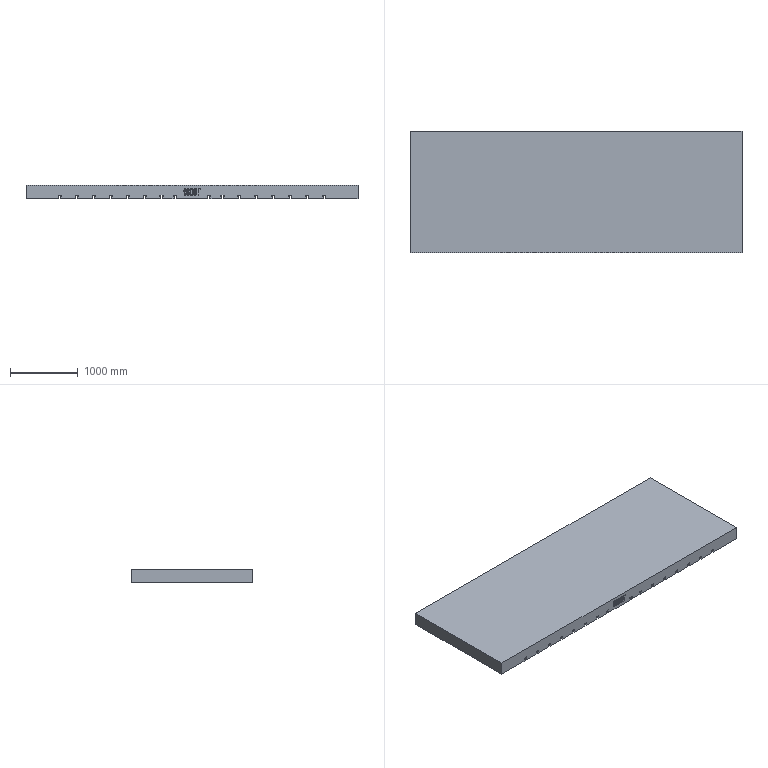Part | STEP file | lll_id3714_x_t | 1 solid | 237 faces | box 4900 x 1800 x 200 mm | volume 1712595456 mm3 | plane 223 | other 14